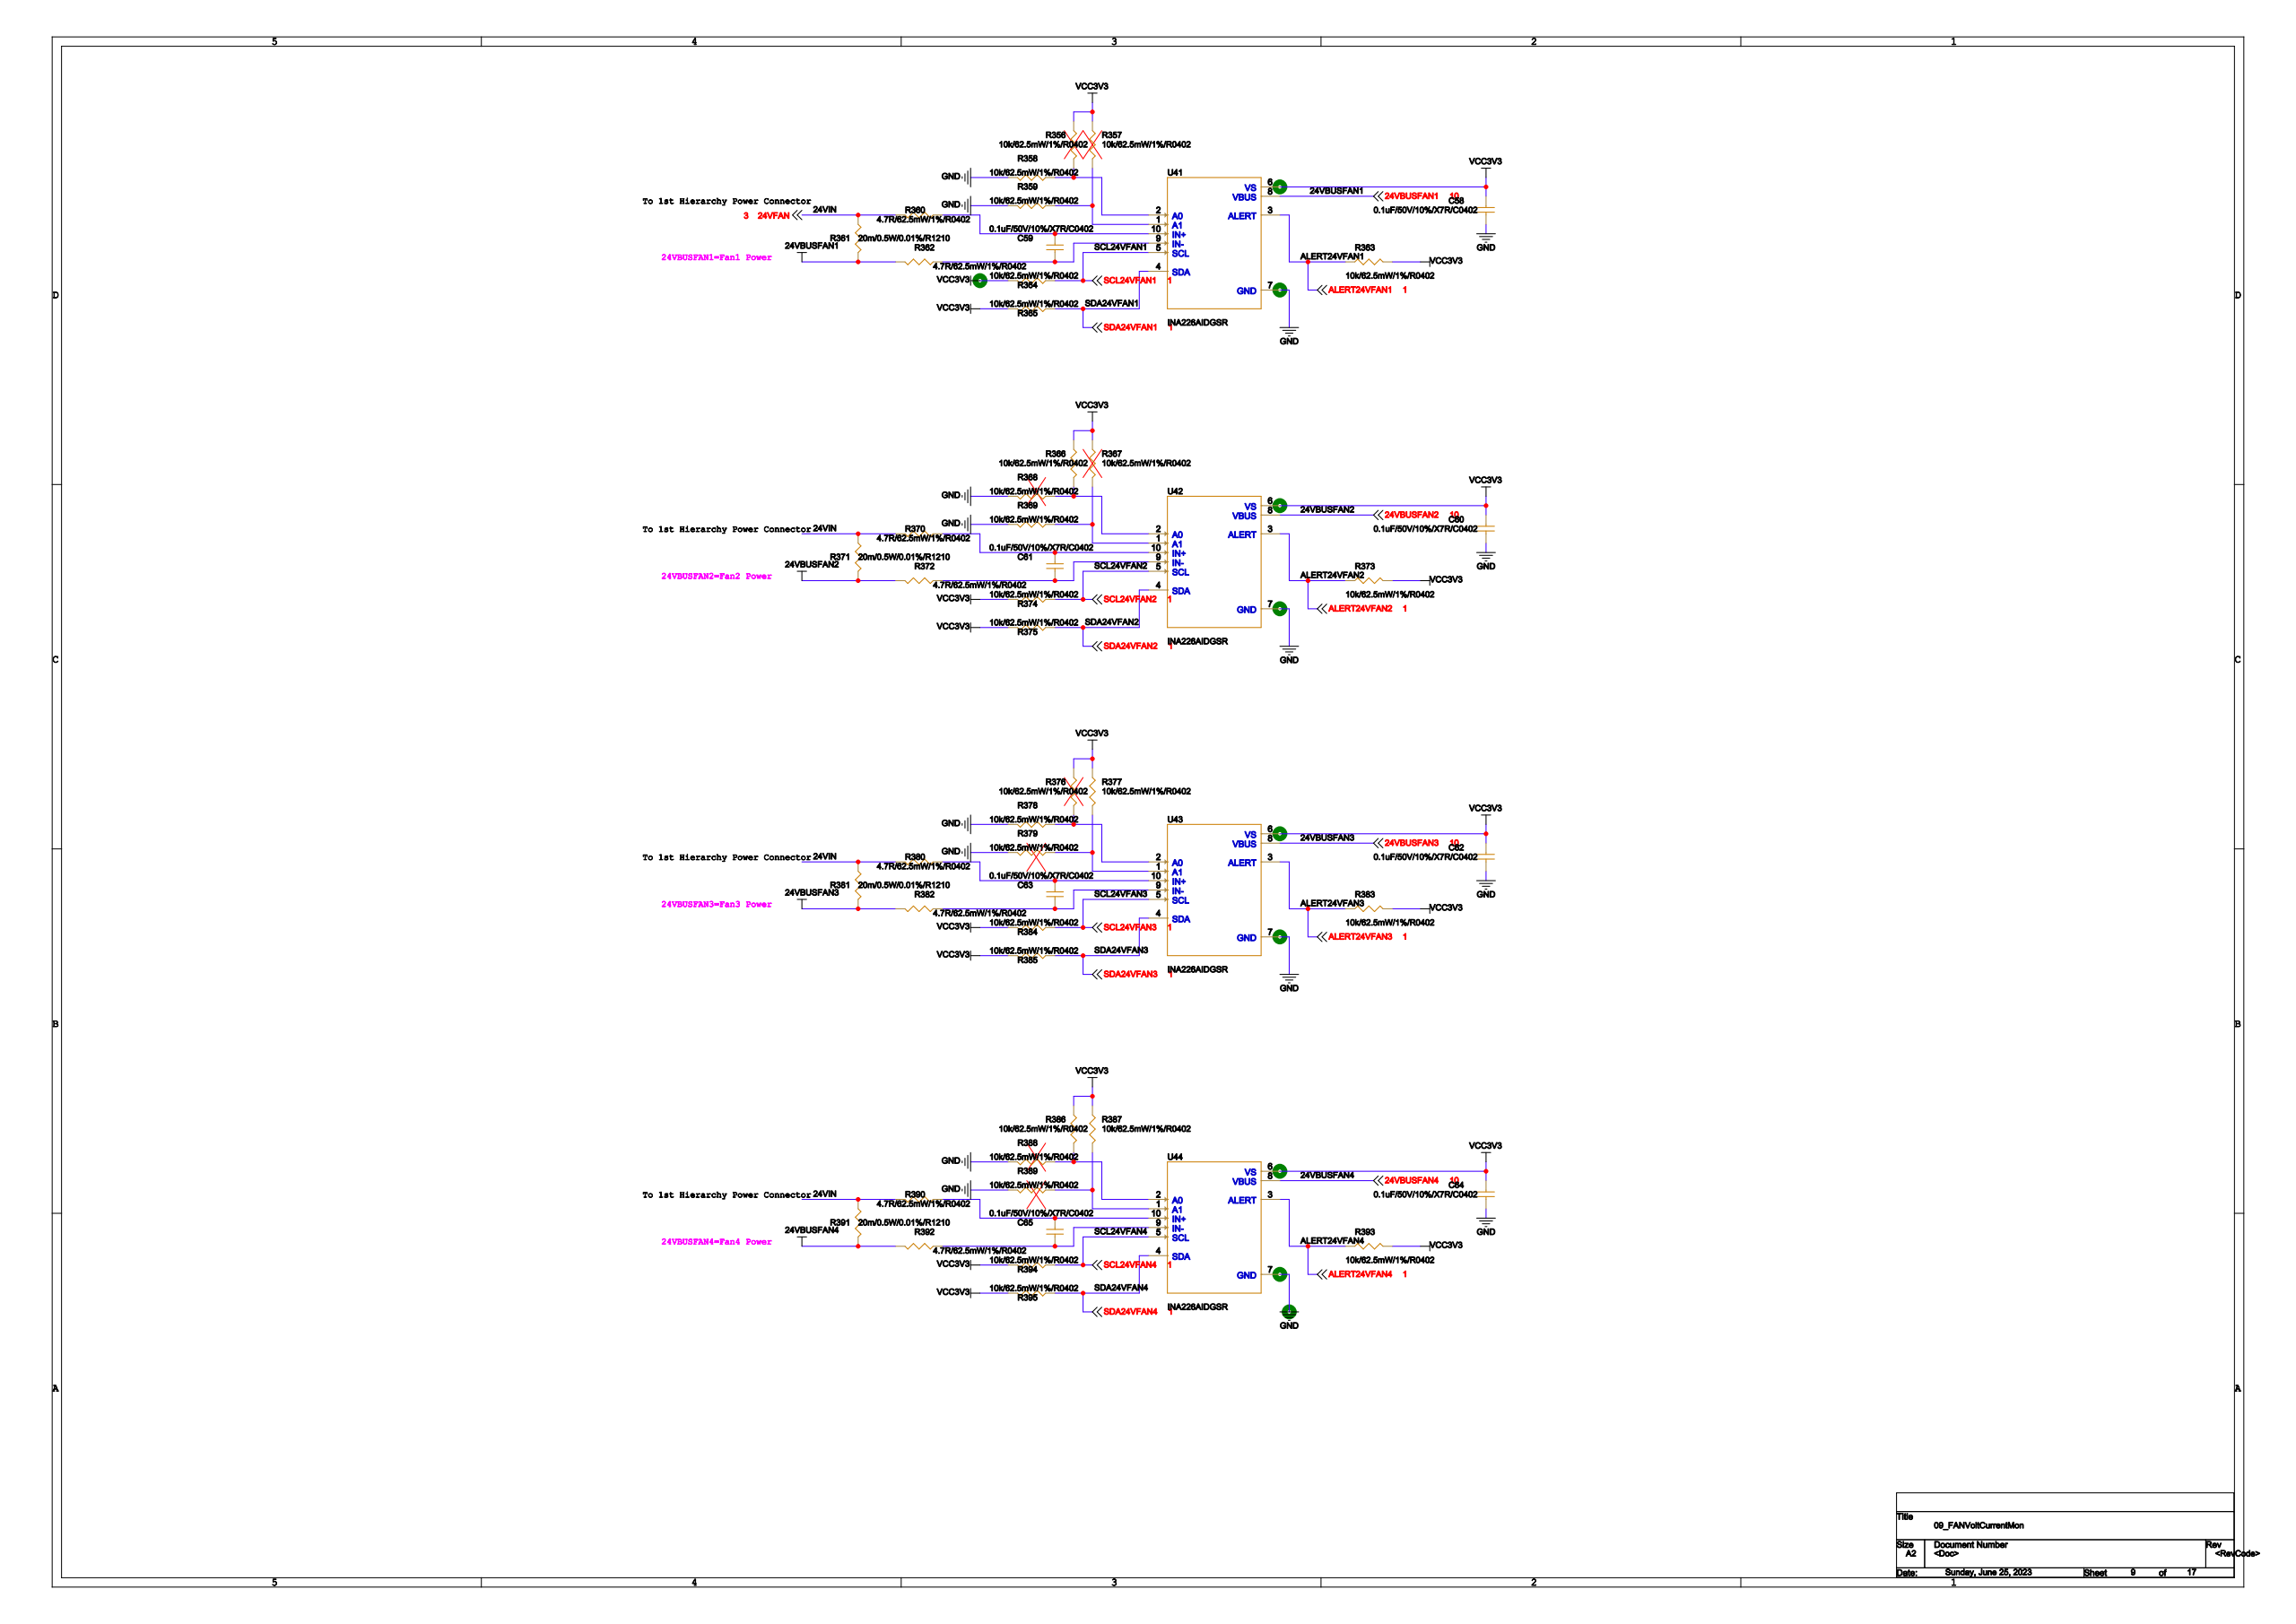Circuit board | Cadence Allegro | 1997 parts | 1536 nets | one sheet of the schematic
Parts on this sheet (reference | value | footprint):
C58 | 0.1uF/50V/10%/X7R/C0402 | 0402
C59 | 0.1uF/50V/10%/X7R/C0402 | 0402
C60 | 0.1uF/50V/10%/X7R/C0402 | 0402
C61 | 0.1uF/50V/10%/X7R/C0402 | 0402
C62 | 0.1uF/50V/10%/X7R/C0402 | 0402
C63 | 0.1uF/50V/10%/X7R/C0402 | 0402
C64 | 0.1uF/50V/10%/X7R/C0402 | 0402
C65 | 0.1uF/50V/10%/X7R/C0402 | 0402
R356 | 10k/62.5mW/1%/R0402 | 0402
R357 | 10k/62.5mW/1%/R0402 | 0402
R358 | 10k/62.5mW/1%/R0402 | 0402
R359 | 10k/62.5mW/1%/R0402 | 0402
R360 | 4.7R/62.5mW/1%/R0402 | 0402
R361 | 20m/0.5W/0.01%/R1210 | 1210
R362 | 4.7R/62.5mW/1%/R0402 | 0402
R363 | 10k/62.5mW/1%/R0402 | 0402
R364 | 10k/62.5mW/1%/R0402 | 0402
R365 | 10k/62.5mW/1%/R0402 | 0402
R366 | 10k/62.5mW/1%/R0402 | 0402
R367 | 10k/62.5mW/1%/R0402 | 0402
R368 | 10k/62.5mW/1%/R0402 | 0402
R369 | 10k/62.5mW/1%/R0402 | 0402
R370 | 4.7R/62.5mW/1%/R0402 | 0402
R371 | 20m/0.5W/0.01%/R1210 | 1210
R372 | 4.7R/62.5mW/1%/R0402 | 0402
R373 | 10k/62.5mW/1%/R0402 | 0402
R374 | 10k/62.5mW/1%/R0402 | 0402
R375 | 10k/62.5mW/1%/R0402 | 0402
R376 | 10k/62.5mW/1%/R0402 | 0402
R377 | 10k/62.5mW/1%/R0402 | 0402
R378 | 10k/62.5mW/1%/R0402 | 0402
R379 | 10k/62.5mW/1%/R0402 | 0402
R380 | 4.7R/62.5mW/1%/R0402 | 0402
R381 | 20m/0.5W/0.01%/R1210 | 1210
R382 | 4.7R/62.5mW/1%/R0402 | 0402
R383 | 10k/62.5mW/1%/R0402 | 0402
R384 | 10k/62.5mW/1%/R0402 | 0402
R385 | 10k/62.5mW/1%/R0402 | 0402
R386 | 10k/62.5mW/1%/R0402 | 0402
R387 | 10k/62.5mW/1%/R0402 | 0402
R388 | 10k/62.5mW/1%/R0402 | 0402
R389 | 10k/62.5mW/1%/R0402 | 0402
R390 | 4.7R/62.5mW/1%/R0402 | 0402
R391 | 20m/0.5W/0.01%/R1210 | 1210
R392 | 4.7R/62.5mW/1%/R0402 | 0402
R393 | 10k/62.5mW/1%/R0402 | 0402
R394 | 10k/62.5mW/1%/R0402 | 0402
R395 | 10k/62.5mW/1%/R0402 | 0402
U41 | INA226AIDGSR | SOP50P490X110-10N
U42 | INA226AIDGSR | SOP50P490X110-10N
U43 | INA226AIDGSR | SOP50P490X110-10N
U44 | INA226AIDGSR | SOP50P490X110-10N
Nets of these parts (net: part-pin ...):
3.3V: C58-1 C60-1 C62-1 C64-1 R356-1 R357-1 R363-2 R364-2 R365-2 R366-1 R367-1 R373-2 R374-2 R375-2 R376-1 R377-1 R383-2 R384-2 R385-2 R386-1 R387-1 R393-2 R394-2 R395-2 U41-6 U42-6 U43-6 U44-6
AGND: C58-2 C60-2 C62-2 C64-2 R358-2 R359-2 R368-2 R369-2 R378-2 R379-2 R388-2 R389-2 U41-7 U42-7 U43-7 U44-7
SCL24VFAN1: R364-1 U41-5
SDA24VFAN1: R365-1 U41-4
ALERT24VFAN1: R363-1 U41-3
SCL24VFAN2: R374-1 U42-5
SDA24VFAN2: R375-1 U42-4
ALERT24VFAN2: R373-1 U42-3
SCL24VFAN3: R384-1 U43-5
SDA24VFAN3: R385-1 U43-4
ALERT24VFAN3: R383-1 U43-3
ALERT24VFAN4: R393-1 U44-3
SCL24VFAN4: R394-1 U44-5
SDA24VFAN4: R395-1 U44-4
24VBUSFAN1: R361-2 R362-2 U41-8
24VBUSFAN4: R391-2 R392-2 U44-8
24VBUSFAN2: R371-2 R372-2 U42-8
24VBUSFAN3: R381-2 R382-2 U43-8
24VFAN: R360-2 R361-1 R370-2 R371-1 R380-2 R381-1 R390-2 R391-1
N23136700: C59-1 R360-1 U41-10
N23136726: C59-2 R362-1 U41-9
N23189446: C61-1 R370-1 U42-10
N23189612: C61-2 R372-1 U42-9
N23190079: C63-1 R380-1 U43-10
N23190245: C63-2 R382-1 U43-9
N23190745: C65-1 R390-1 U44-10
N23190911: C65-2 R392-1 U44-9
N23136475: R356-2 R358-1 U41-2
N23136485: R357-2 R359-1 U41-1
N23189541: R366-2 R368-1 U42-2
N23189547: R367-2 R369-1 U42-1
N23190174: R376-2 R378-1 U43-2
N23190180: R377-2 R379-1 U43-1
N23190840: R386-2 R388-1 U44-2
N23190846: R387-2 R389-1 U44-1